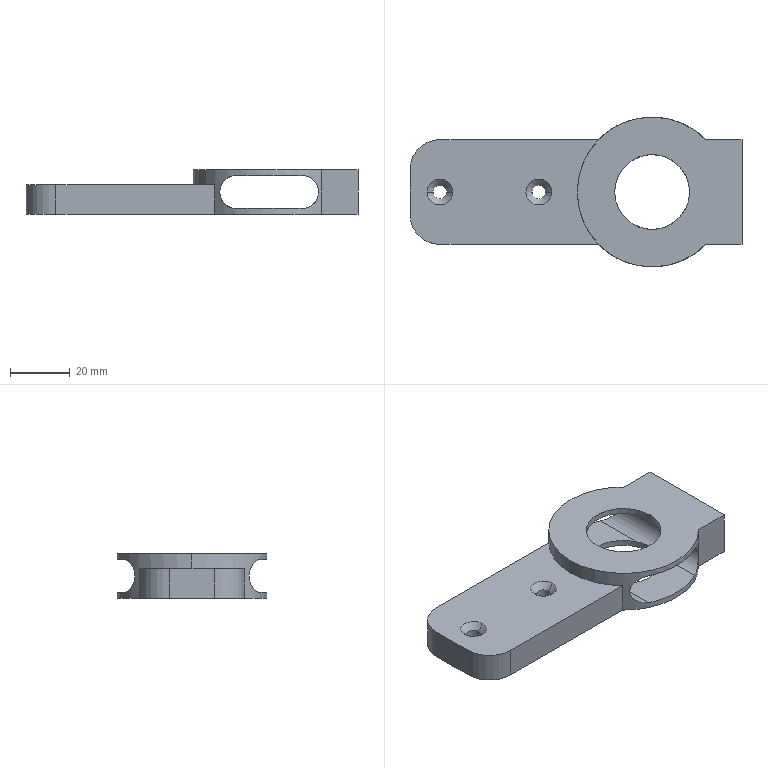Part | STEP file | 1 solid | 31 faces | box 110.854 x 50 x 15 mm | volume 35082 mm3 | cylinder 14 | plane 13 | cone 4 | commonest cylinder face diameters 4.5 x4 25 x4 11 x2 20 x2 50 x2